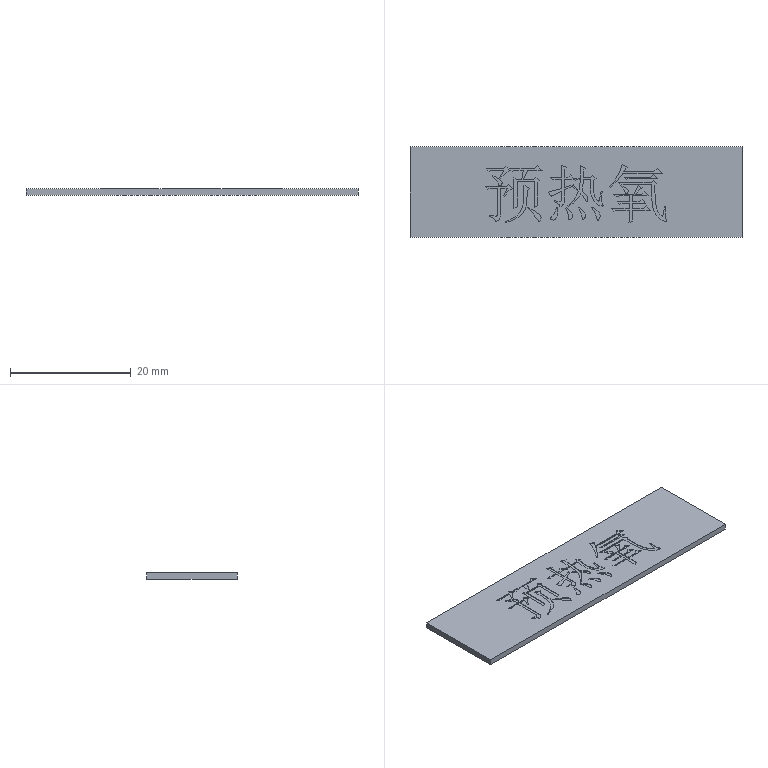Part | STEP file | HXGR200008-06-02-06 | 1 solid | 228 faces | box 55 x 15 x 1 mm | volume 818.976 mm3 | plane 143 | spline 85